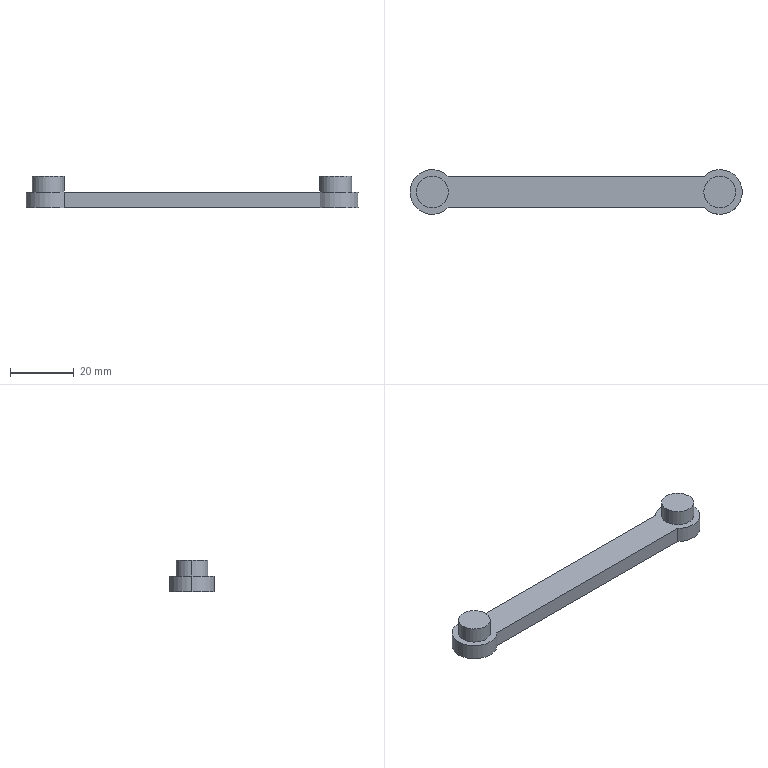Part | SolidWorks | features Boss 1, Extrusion 1 | 1 solid | 13 faces | box 104 x 14 x 10 mm | volume 6190 mm3 | cylinder 7 | plane 6 | commonest cylinder face diameters 10 x4 14 x3
STEP:
#1=CARTESIAN_POINT('',(95.,0.,10.));
#2=VERTEX_POINT('',#1);
#3=CARTESIAN_POINT('',(85.,0.,10.));
#4=VERTEX_POINT('',#3);
#5=CARTESIAN_POINT('',(90.,0.,10.));
#6=DIRECTION('',(0.,0.,1.));
#7=DIRECTION('',(1.,0.,0.));
#8=AXIS2_PLACEMENT_3D('',#5,#6,#7);
#9=CIRCLE('',#8,5.);
#10=EDGE_CURVE('',#2,#4,#9,.T.);
#11=ORIENTED_EDGE('',*,*,#10,.F.);
#12=CARTESIAN_POINT('',(95.,0.,5.));
#13=VERTEX_POINT('',#12);
#14=CARTESIAN_POINT('',(95.,0.,10.));
#15=DIRECTION('',(0.,0.,-1.));
#16=VECTOR('',#15,1000.);
#17=LINE('',#14,#16);
#18=EDGE_CURVE('',#2,#13,#17,.T.);
#19=ORIENTED_EDGE('',*,*,#18,.T.);
#20=CARTESIAN_POINT('',(85.,0.,5.));
#21=VERTEX_POINT('',#20);
#22=CARTESIAN_POINT('',(90.,0.,5.));
#23=DIRECTION('',(0.,0.,1.));
#24=DIRECTION('',(1.,0.,0.));
#25=AXIS2_PLACEMENT_3D('',#22,#23,#24);
#26=CIRCLE('',#25,5.);
#27=EDGE_CURVE('',#13,#21,#26,.T.);
#28=ORIENTED_EDGE('',*,*,#27,.T.);
#29=CARTESIAN_POINT('',(85.,0.,10.));
#30=DIRECTION('',(0.,0.,-1.));
#31=VECTOR('',#30,1000.);
#32=LINE('',#29,#31);
#33=EDGE_CURVE('',#4,#21,#32,.T.);
#34=ORIENTED_EDGE('',*,*,#33,.F.);
#35=EDGE_LOOP('',(#11,#19,#28,#34));
#36=FACE_OUTER_BOUND('',#35,.T.);
#37=CARTESIAN_POINT('',(90.,0.,10.));
#38=DIRECTION('',(0.,0.,-1.));
#39=DIRECTION('',(-1.,0.,0.));
#40=AXIS2_PLACEMENT_3D('',#37,#38,#39);
#41=CYLINDRICAL_SURFACE('',#40,5.);
#42=ADVANCED_FACE('',(#36),#41,.T.);
#43=CARTESIAN_POINT('',(5.,0.,10.));
#44=VERTEX_POINT('',#43);
#45=CARTESIAN_POINT('',(-5.,0.,10.));
#46=VERTEX_POINT('',#45);
#47=CARTESIAN_POINT('',(0.,0.,10.));
#48=DIRECTION('',(0.,0.,1.));
#49=DIRECTION('',(1.,0.,0.));
#50=AXIS2_PLACEMENT_3D('',#47,#48,#49);
#51=CIRCLE('',#50,5.);
#52=EDGE_CURVE('',#44,#46,#51,.T.);
#53=ORIENTED_EDGE('',*,*,#52,.F.);
#54=CARTESIAN_POINT('',(5.,0.,5.));
#55=VERTEX_POINT('',#54);
#56=CARTESIAN_POINT('',(5.,0.,10.));
#57=DIRECTION('',(0.,0.,-1.));
#58=VECTOR('',#57,1000.);
#59=LINE('',#56,#58);
#60=EDGE_CURVE('',#44,#55,#59,.T.);
#61=ORIENTED_EDGE('',*,*,#60,.T.);
#62=CARTESIAN_POINT('',(-5.,0.,5.));
#63=VERTEX_POINT('',#62);
#64=CARTESIAN_POINT('',(0.,0.,5.));
#65=DIRECTION('',(0.,0.,1.));
#66=DIRECTION('',(1.,0.,0.));
#67=AXIS2_PLACEMENT_3D('',#64,#65,#66);
#68=CIRCLE('',#67,5.);
#69=EDGE_CURVE('',#55,#63,#68,.T.);
#70=ORIENTED_EDGE('',*,*,#69,.T.);
#71=CARTESIAN_POINT('',(-5.,0.,10.));
#72=DIRECTION('',(0.,0.,-1.));
#73=VECTOR('',#72,1000.);
#74=LINE('',#71,#73);
#75=EDGE_CURVE('',#46,#63,#74,.T.);
#76=ORIENTED_EDGE('',*,*,#75,.F.);
#77=EDGE_LOOP('',(#53,#61,#70,#76));
#78=FACE_OUTER_BOUND('',#77,.T.);
#79=CARTESIAN_POINT('',(0.,0.,10.));
#80=DIRECTION('',(0.,0.,-1.));
#81=DIRECTION('',(-1.,0.,0.));
#82=AXIS2_PLACEMENT_3D('',#79,#80,#81);
#83=CYLINDRICAL_SURFACE('',#82,5.);
#84=ADVANCED_FACE('',(#78),#83,.T.);
#85=CARTESIAN_POINT('',(-7.,0.,5.));
#86=VERTEX_POINT('',#85);
#87=CARTESIAN_POINT('',(4.899,-5.,5.));
#88=VERTEX_POINT('',#87);
#89=CARTESIAN_POINT('',(0.,0.,5.));
#90=DIRECTION('',(0.,0.,1.));
#91=DIRECTION('',(1.,0.,0.));
#92=AXIS2_PLACEMENT_3D('',#89,#90,#91);
#93=CIRCLE('',#92,7.);
#94=EDGE_CURVE('',#86,#88,#93,.T.);
#95=ORIENTED_EDGE('',*,*,#94,.F.);
#96=CARTESIAN_POINT('',(-7.,0.,0.));
#97=VERTEX_POINT('',#96);
#98=CARTESIAN_POINT('',(-7.,0.,5.));
#99=DIRECTION('',(0.,0.,-1.));
#100=VECTOR('',#99,1000.);
#101=LINE('',#98,#100);
#102=EDGE_CURVE('',#86,#97,#101,.T.);
#103=ORIENTED_EDGE('',*,*,#102,.T.);
#104=CARTESIAN_POINT('',(4.899,-5.,0.));
#105=VERTEX_POINT('',#104);
#106=CARTESIAN_POINT('',(0.,0.,0.));
#107=DIRECTION('',(0.,0.,1.));
#108=DIRECTION('',(1.,0.,0.));
#109=AXIS2_PLACEMENT_3D('',#106,#107,#108);
#110=CIRCLE('',#109,7.);
#111=EDGE_CURVE('',#97,#105,#110,.T.);
#112=ORIENTED_EDGE('',*,*,#111,.T.);
#113=CARTESIAN_POINT('',(4.899,-5.,5.));
#114=DIRECTION('',(0.,0.,-1.));
#115=VECTOR('',#114,1000.);
#116=LINE('',#113,#115);
#117=EDGE_CURVE('',#88,#105,#116,.T.);
#118=ORIENTED_EDGE('',*,*,#117,.F.);
#119=EDGE_LOOP('',(#95,#103,#112,#118));
#120=FACE_OUTER_BOUND('',#119,.T.);
#121=CARTESIAN_POINT('',(0.,0.,5.));
#122=DIRECTION('',(0.,0.,-1.));
#123=DIRECTION('',(-1.,0.,0.));
#124=AXIS2_PLACEMENT_3D('',#121,#122,#123);
#125=CYLINDRICAL_SURFACE('',#124,7.);
#126=ADVANCED_FACE('',(#120),#125,.T.);
#127=CARTESIAN_POINT('',(0.,0.,5.));
#128=DIRECTION('',(0.,0.,1.));
#129=DIRECTION('',(1.,0.,0.));
#130=AXIS2_PLACEMENT_3D('',#127,#128,#129);
#131=CIRCLE('',#130,5.);
#132=EDGE_CURVE('',#63,#55,#131,.T.);
#133=ORIENTED_EDGE('',*,*,#132,.F.);
#134=ORIENTED_EDGE('',*,*,#69,.F.);
#135=EDGE_LOOP('',(#133,#134));
#136=FACE_BOUND('',#135,.T.);
#137=CARTESIAN_POINT('',(4.899,5.,5.));
#138=VERTEX_POINT('',#137);
#139=CARTESIAN_POINT('',(0.,0.,5.));
#140=DIRECTION('',(0.,0.,1.));
#141=DIRECTION('',(1.,0.,0.));
#142=AXIS2_PLACEMENT_3D('',#139,#140,#141);
#143=CIRCLE('',#142,7.);
#144=EDGE_CURVE('',#138,#86,#143,.T.);
#145=ORIENTED_EDGE('',*,*,#144,.T.);
#146=ORIENTED_EDGE('',*,*,#94,.T.);
#147=CARTESIAN_POINT('',(85.101,-5.,5.));
#148=VERTEX_POINT('',#147);
#149=CARTESIAN_POINT('',(4.899,-5.,5.));
#150=DIRECTION('',(1.,0.,0.));
#151=VECTOR('',#150,1000.);
#152=LINE('',#149,#151);
#153=EDGE_CURVE('',#88,#148,#152,.T.);
#154=ORIENTED_EDGE('',*,*,#153,.T.);
#155=CARTESIAN_POINT('',(85.101,5.,5.));
#156=VERTEX_POINT('',#155);
#157=CARTESIAN_POINT('',(90.,0.,5.));
#158=DIRECTION('',(0.,0.,1.));
#159=DIRECTION('',(1.,0.,0.));
#160=AXIS2_PLACEMENT_3D('',#157,#158,#159);
#161=CIRCLE('',#160,7.);
#162=EDGE_CURVE('',#148,#156,#161,.T.);
#163=ORIENTED_EDGE('',*,*,#162,.T.);
#164=CARTESIAN_POINT('',(4.899,5.,5.));
#165=DIRECTION('',(-1.,0.,0.));
#166=VECTOR('',#165,1000.);
#167=LINE('',#164,#166);
#168=EDGE_CURVE('',#156,#138,#167,.T.);
#169=ORIENTED_EDGE('',*,*,#168,.T.);
#170=EDGE_LOOP('',(#145,#146,#154,#163,#169));
#171=FACE_OUTER_BOUND('',#170,.T.);
#172=CARTESIAN_POINT('',(90.,0.,5.));
#173=DIRECTION('',(0.,0.,1.));
#174=DIRECTION('',(1.,0.,0.));
#175=AXIS2_PLACEMENT_3D('',#172,#173,#174);
#176=CIRCLE('',#175,5.);
#177=EDGE_CURVE('',#21,#13,#176,.T.);
#178=ORIENTED_EDGE('',*,*,#177,.F.);
#179=ORIENTED_EDGE('',*,*,#27,.F.);
#180=EDGE_LOOP('',(#178,#179));
#181=FACE_BOUND('',#180,.T.);
#182=CARTESIAN_POINT('',(0.,0.,5.));
#183=DIRECTION('',(0.,0.,1.));
#184=DIRECTION('',(1.,0.,0.));
#185=AXIS2_PLACEMENT_3D('',#182,#183,#184);
#186=PLANE('',#185);
#187=ADVANCED_FACE('',(#136,#171,#181),#186,.T.);
#188=ORIENTED_EDGE('',*,*,#102,.F.);
#189=ORIENTED_EDGE('',*,*,#144,.F.);
#190=CARTESIAN_POINT('',(4.899,5.,0.));
#191=VERTEX_POINT('',#190);
#192=CARTESIAN_POINT('',(4.899,5.,5.));
#193=DIRECTION('',(0.,0.,-1.));
#194=VECTOR('',#193,1000.);
#195=LINE('',#192,#194);
#196=EDGE_CURVE('',#138,#191,#195,.T.);
#197=ORIENTED_EDGE('',*,*,#196,.T.);
#198=CARTESIAN_POINT('',(0.,0.,0.));
#199=DIRECTION('',(0.,0.,1.));
#200=DIRECTION('',(1.,0.,0.));
#201=AXIS2_PLACEMENT_3D('',#198,#199,#200);
#202=CIRCLE('',#201,7.);
#203=EDGE_CURVE('',#191,#97,#202,.T.);
#204=ORIENTED_EDGE('',*,*,#203,.T.);
#205=EDGE_LOOP('',(#188,#189,#197,#204));
#206=FACE_OUTER_BOUND('',#205,.T.);
#207=CARTESIAN_POINT('',(0.,0.,5.));
#208=DIRECTION('',(0.,0.,-1.));
#209=DIRECTION('',(-1.,0.,0.));
#210=AXIS2_PLACEMENT_3D('',#207,#208,#209);
#211=CYLINDRICAL_SURFACE('',#210,7.);
#212=ADVANCED_FACE('',(#206),#211,.T.);
#213=CARTESIAN_POINT('',(85.101,-5.,0.));
#214=VERTEX_POINT('',#213);
#215=CARTESIAN_POINT('',(4.899,-5.,0.));
#216=DIRECTION('',(1.,0.,0.));
#217=VECTOR('',#216,1000.);
#218=LINE('',#215,#217);
#219=EDGE_CURVE('',#105,#214,#218,.T.);
#220=ORIENTED_EDGE('',*,*,#219,.T.);
#221=CARTESIAN_POINT('',(85.101,-5.,5.));
#222=DIRECTION('',(0.,0.,-1.));
#223=VECTOR('',#222,1000.);
#224=LINE('',#221,#223);
#225=EDGE_CURVE('',#148,#214,#224,.T.);
#226=ORIENTED_EDGE('',*,*,#225,.F.);
#227=ORIENTED_EDGE('',*,*,#153,.F.);
#228=ORIENTED_EDGE('',*,*,#117,.T.);
#229=EDGE_LOOP('',(#220,#226,#227,#228));
#230=FACE_OUTER_BOUND('',#229,.T.);
#231=CARTESIAN_POINT('',(4.899,-5.,5.));
#232=DIRECTION('',(0.,1.,0.));
#233=DIRECTION('',(0.,0.,1.));
#234=AXIS2_PLACEMENT_3D('',#231,#232,#233);
#235=PLANE('',#234);
#236=ADVANCED_FACE('',(#230),#235,.F.);
#237=CARTESIAN_POINT('',(85.101,5.,0.));
#238=VERTEX_POINT('',#237);
#239=CARTESIAN_POINT('',(90.,0.,0.));
#240=DIRECTION('',(0.,0.,1.));
#241=DIRECTION('',(1.,0.,0.));
#242=AXIS2_PLACEMENT_3D('',#239,#240,#241);
#243=CIRCLE('',#242,7.);
#244=EDGE_CURVE('',#214,#238,#243,.T.);
#245=ORIENTED_EDGE('',*,*,#244,.T.);
#246=CARTESIAN_POINT('',(85.101,5.,5.));
#247=DIRECTION('',(0.,0.,-1.));
#248=VECTOR('',#247,1000.);
#249=LINE('',#246,#248);
#250=EDGE_CURVE('',#156,#238,#249,.T.);
#251=ORIENTED_EDGE('',*,*,#250,.F.);
#252=ORIENTED_EDGE('',*,*,#162,.F.);
#253=ORIENTED_EDGE('',*,*,#225,.T.);
#254=EDGE_LOOP('',(#245,#251,#252,#253));
#255=FACE_OUTER_BOUND('',#254,.T.);
#256=CARTESIAN_POINT('',(90.,0.,5.));
#257=DIRECTION('',(0.,0.,-1.));
#258=DIRECTION('',(-1.,0.,0.));
#259=AXIS2_PLACEMENT_3D('',#256,#257,#258);
#260=CYLINDRICAL_SURFACE('',#259,7.);
#261=ADVANCED_FACE('',(#255),#260,.T.);
#262=CARTESIAN_POINT('',(4.899,5.,0.));
#263=DIRECTION('',(-1.,0.,0.));
#264=VECTOR('',#263,1000.);
#265=LINE('',#262,#264);
#266=EDGE_CURVE('',#238,#191,#265,.T.);
#267=ORIENTED_EDGE('',*,*,#266,.T.);
#268=ORIENTED_EDGE('',*,*,#196,.F.);
#269=ORIENTED_EDGE('',*,*,#168,.F.);
#270=ORIENTED_EDGE('',*,*,#250,.T.);
#271=EDGE_LOOP('',(#267,#268,#269,#270));
#272=FACE_OUTER_BOUND('',#271,.T.);
#273=CARTESIAN_POINT('',(4.899,5.,5.));
#274=DIRECTION('',(0.,-1.,0.));
#275=DIRECTION('',(0.,0.,-1.));
#276=AXIS2_PLACEMENT_3D('',#273,#274,#275);
#277=PLANE('',#276);
#278=ADVANCED_FACE('',(#272),#277,.F.);
#279=ORIENTED_EDGE('',*,*,#203,.F.);
#280=ORIENTED_EDGE('',*,*,#266,.F.);
#281=ORIENTED_EDGE('',*,*,#244,.F.);
#282=ORIENTED_EDGE('',*,*,#219,.F.);
#283=ORIENTED_EDGE('',*,*,#111,.F.);
#284=EDGE_LOOP('',(#279,#280,#281,#282,#283));
#285=FACE_OUTER_BOUND('',#284,.T.);
#286=CARTESIAN_POINT('',(0.,0.,0.));
#287=DIRECTION('',(0.,0.,1.));
#288=DIRECTION('',(1.,0.,0.));
#289=AXIS2_PLACEMENT_3D('',#286,#287,#288);
#290=PLANE('',#289);
#291=ADVANCED_FACE('',(#285),#290,.F.);
#292=ORIENTED_EDGE('',*,*,#60,.F.);
#293=CARTESIAN_POINT('',(0.,0.,10.));
#294=DIRECTION('',(0.,0.,1.));
#295=DIRECTION('',(1.,0.,0.));
#296=AXIS2_PLACEMENT_3D('',#293,#294,#295);
#297=CIRCLE('',#296,5.);
#298=EDGE_CURVE('',#46,#44,#297,.T.);
#299=ORIENTED_EDGE('',*,*,#298,.F.);
#300=ORIENTED_EDGE('',*,*,#75,.T.);
#301=ORIENTED_EDGE('',*,*,#132,.T.);
#302=EDGE_LOOP('',(#292,#299,#300,#301));
#303=FACE_OUTER_BOUND('',#302,.T.);
#304=CARTESIAN_POINT('',(0.,0.,10.));
#305=DIRECTION('',(0.,0.,-1.));
#306=DIRECTION('',(-1.,0.,0.));
#307=AXIS2_PLACEMENT_3D('',#304,#305,#306);
#308=CYLINDRICAL_SURFACE('',#307,5.);
#309=ADVANCED_FACE('',(#303),#308,.T.);
#310=ORIENTED_EDGE('',*,*,#298,.T.);
#311=ORIENTED_EDGE('',*,*,#52,.T.);
#312=EDGE_LOOP('',(#310,#311));
#313=FACE_OUTER_BOUND('',#312,.T.);
#314=CARTESIAN_POINT('',(0.,0.,10.));
#315=DIRECTION('',(0.,0.,1.));
#316=DIRECTION('',(1.,0.,0.));
#317=AXIS2_PLACEMENT_3D('',#314,#315,#316);
#318=PLANE('',#317);
#319=ADVANCED_FACE('',(#313),#318,.T.);
#320=ORIENTED_EDGE('',*,*,#18,.F.);
#321=CARTESIAN_POINT('',(90.,0.,10.));
#322=DIRECTION('',(0.,0.,1.));
#323=DIRECTION('',(1.,0.,0.));
#324=AXIS2_PLACEMENT_3D('',#321,#322,#323);
#325=CIRCLE('',#324,5.);
#326=EDGE_CURVE('',#4,#2,#325,.T.);
#327=ORIENTED_EDGE('',*,*,#326,.F.);
#328=ORIENTED_EDGE('',*,*,#33,.T.);
#329=ORIENTED_EDGE('',*,*,#177,.T.);
#330=EDGE_LOOP('',(#320,#327,#328,#329));
#331=FACE_OUTER_BOUND('',#330,.T.);
#332=CARTESIAN_POINT('',(90.,0.,10.));
#333=DIRECTION('',(0.,0.,-1.));
#334=DIRECTION('',(-1.,0.,0.));
#335=AXIS2_PLACEMENT_3D('',#332,#333,#334);
#336=CYLINDRICAL_SURFACE('',#335,5.);
#337=ADVANCED_FACE('',(#331),#336,.T.);
#338=ORIENTED_EDGE('',*,*,#326,.T.);
#339=ORIENTED_EDGE('',*,*,#10,.T.);
#340=EDGE_LOOP('',(#338,#339));
#341=FACE_OUTER_BOUND('',#340,.T.);
#342=CARTESIAN_POINT('',(90.,0.,10.));
#343=DIRECTION('',(0.,0.,1.));
#344=DIRECTION('',(1.,0.,0.));
#345=AXIS2_PLACEMENT_3D('',#342,#343,#344);
#346=PLANE('',#345);
#347=ADVANCED_FACE('',(#341),#346,.T.);
#348=CLOSED_SHELL('',(#42,#84,#126,#187,#212,#236,#261,#278,#291,#309,#319,#337,#347));
#349=MANIFOLD_SOLID_BREP('',#348);
#350=CARTESIAN_POINT('',(0.,0.,0.));
#351=DIRECTION('',(0.,0.,1.));
#352=DIRECTION('',(1.,0.,0.));
#353=AXIS2_PLACEMENT_3D('',#350,#351,#352);
#354=(LENGTH_UNIT()NAMED_UNIT(*)SI_UNIT(.MILLI.,.METRE.));
#355=UNCERTAINTY_MEASURE_WITH_UNIT(LENGTH_MEASURE(0.00001),#354,'','');
#356=(NAMED_UNIT(*)PLANE_ANGLE_UNIT()SI_UNIT($,.RADIAN.));
#357=(NAMED_UNIT(*)SI_UNIT($,.STERADIAN.)SOLID_ANGLE_UNIT());
#358=(GEOMETRIC_REPRESENTATION_CONTEXT(3)GLOBAL_UNCERTAINTY_ASSIGNED_CONTEXT((#355))GLOBAL_UNIT_ASSIGNED_CONTEXT((#354,#356,#357))REPRESENTATION_CONTEXT('',''));
#359=ADVANCED_BREP_SHAPE_REPRESENTATION('',(#349,#353),#358);